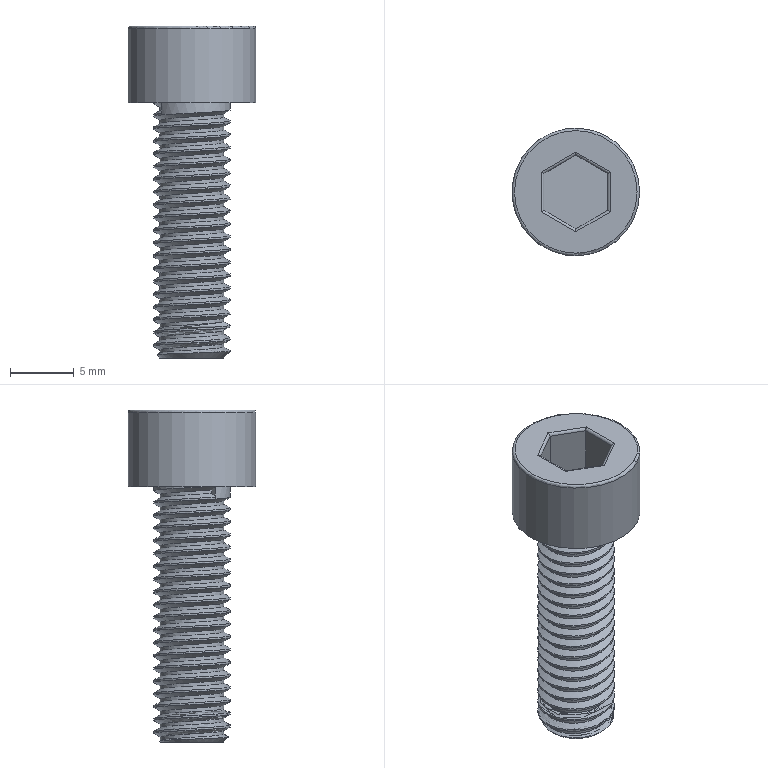Part | STEP file | Tube feed_id1530_x_t | 1 solid | 26 faces | box 10 x 10 x 26 mm | volume 852.808 mm3 | plane 12 | cylinder 9 | spline 3 | torus 1 | cone 1 | commonest cylinder face diameters 0.4 x6 5 x1 6 x1 10 x1